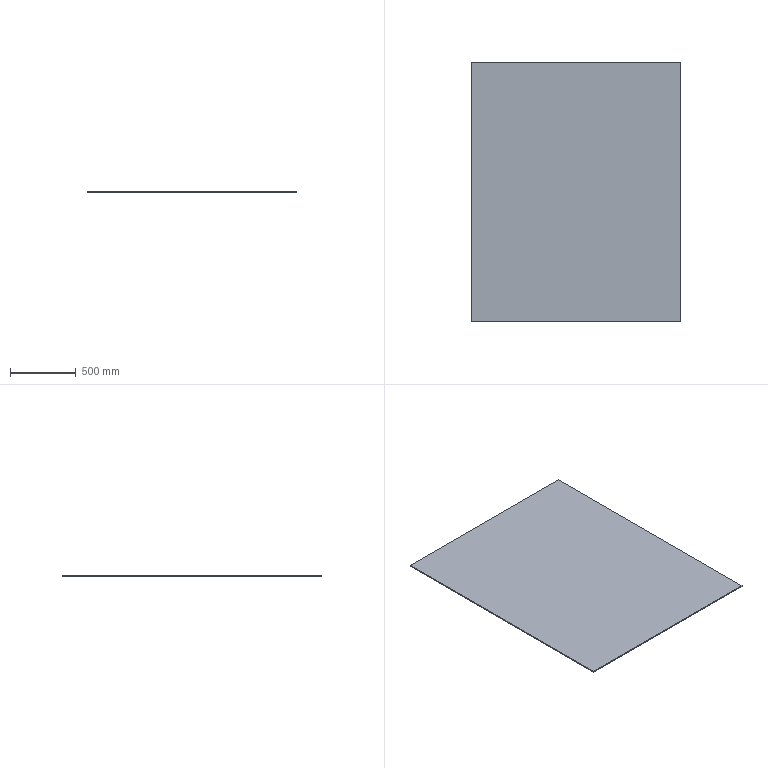Part | SolidWorks | features BaseBody 1, MoveFace 1 | 1 solid | 6 faces | box 1590 x 1968 x 8 mm | volume 25032960 mm3 | plane 6
STEP:
#1=CARTESIAN_POINT('',(0.,2.,0.));
#2=VERTEX_POINT('',#1);
#3=CARTESIAN_POINT('',(1590.,2.,0.));
#4=VERTEX_POINT('',#3);
#5=CARTESIAN_POINT('',(0.,2.,0.));
#6=DIRECTION('',(1.,0.,0.));
#7=VECTOR('',#6,1000.);
#8=LINE('',#5,#7);
#9=EDGE_CURVE('',#2,#4,#8,.T.);
#10=ORIENTED_EDGE('',*,*,#9,.F.);
#11=CARTESIAN_POINT('',(0.,1970.,0.));
#12=VERTEX_POINT('',#11);
#13=CARTESIAN_POINT('',(0.,1970.,0.));
#14=DIRECTION('',(0.,-1.,0.));
#15=VECTOR('',#14,1000.);
#16=LINE('',#13,#15);
#17=EDGE_CURVE('',#12,#2,#16,.T.);
#18=ORIENTED_EDGE('',*,*,#17,.F.);
#19=CARTESIAN_POINT('',(1590.,1970.,0.));
#20=VERTEX_POINT('',#19);
#21=CARTESIAN_POINT('',(1590.,1970.,0.));
#22=DIRECTION('',(-1.,0.,0.));
#23=VECTOR('',#22,1000.);
#24=LINE('',#21,#23);
#25=EDGE_CURVE('',#20,#12,#24,.T.);
#26=ORIENTED_EDGE('',*,*,#25,.F.);
#27=CARTESIAN_POINT('',(1590.,0.,0.));
#28=DIRECTION('',(0.,1.,0.));
#29=VECTOR('',#28,1000.);
#30=LINE('',#27,#29);
#31=EDGE_CURVE('',#4,#20,#30,.T.);
#32=ORIENTED_EDGE('',*,*,#31,.F.);
#33=EDGE_LOOP('',(#10,#18,#26,#32));
#34=FACE_OUTER_BOUND('',#33,.T.);
#35=CARTESIAN_POINT('',(795.,985.,0.));
#36=DIRECTION('',(0.,0.,1.));
#37=DIRECTION('',(1.,0.,0.));
#38=AXIS2_PLACEMENT_3D('',#35,#36,#37);
#39=PLANE('',#38);
#40=ADVANCED_FACE('',(#34),#39,.F.);
#41=CARTESIAN_POINT('',(0.,2.,8.));
#42=VERTEX_POINT('',#41);
#43=CARTESIAN_POINT('',(1590.,2.,8.));
#44=VERTEX_POINT('',#43);
#45=CARTESIAN_POINT('',(0.,2.,8.));
#46=DIRECTION('',(1.,0.,0.));
#47=VECTOR('',#46,1000.);
#48=LINE('',#45,#47);
#49=EDGE_CURVE('',#42,#44,#48,.T.);
#50=ORIENTED_EDGE('',*,*,#49,.T.);
#51=CARTESIAN_POINT('',(1590.,1970.,8.));
#52=VERTEX_POINT('',#51);
#53=CARTESIAN_POINT('',(1590.,0.,8.));
#54=DIRECTION('',(0.,1.,0.));
#55=VECTOR('',#54,1000.);
#56=LINE('',#53,#55);
#57=EDGE_CURVE('',#44,#52,#56,.T.);
#58=ORIENTED_EDGE('',*,*,#57,.T.);
#59=CARTESIAN_POINT('',(0.,1970.,8.));
#60=VERTEX_POINT('',#59);
#61=CARTESIAN_POINT('',(1590.,1970.,8.));
#62=DIRECTION('',(-1.,0.,0.));
#63=VECTOR('',#62,1000.);
#64=LINE('',#61,#63);
#65=EDGE_CURVE('',#52,#60,#64,.T.);
#66=ORIENTED_EDGE('',*,*,#65,.T.);
#67=CARTESIAN_POINT('',(0.,1970.,8.));
#68=DIRECTION('',(0.,-1.,0.));
#69=VECTOR('',#68,1000.);
#70=LINE('',#67,#69);
#71=EDGE_CURVE('',#60,#42,#70,.T.);
#72=ORIENTED_EDGE('',*,*,#71,.T.);
#73=EDGE_LOOP('',(#50,#58,#66,#72));
#74=FACE_OUTER_BOUND('',#73,.T.);
#75=CARTESIAN_POINT('',(795.,985.,8.));
#76=DIRECTION('',(0.,0.,1.));
#77=DIRECTION('',(1.,0.,0.));
#78=AXIS2_PLACEMENT_3D('',#75,#76,#77);
#79=PLANE('',#78);
#80=ADVANCED_FACE('',(#74),#79,.T.);
#81=ORIENTED_EDGE('',*,*,#9,.T.);
#82=CARTESIAN_POINT('',(1590.,2.,0.));
#83=DIRECTION('',(0.,0.,1.));
#84=VECTOR('',#83,1000.);
#85=LINE('',#82,#84);
#86=EDGE_CURVE('',#4,#44,#85,.T.);
#87=ORIENTED_EDGE('',*,*,#86,.T.);
#88=ORIENTED_EDGE('',*,*,#49,.F.);
#89=CARTESIAN_POINT('',(0.,2.,0.));
#90=DIRECTION('',(0.,0.,1.));
#91=VECTOR('',#90,1000.);
#92=LINE('',#89,#91);
#93=EDGE_CURVE('',#2,#42,#92,.T.);
#94=ORIENTED_EDGE('',*,*,#93,.F.);
#95=EDGE_LOOP('',(#81,#87,#88,#94));
#96=FACE_OUTER_BOUND('',#95,.T.);
#97=CARTESIAN_POINT('',(0.,2.,0.));
#98=DIRECTION('',(0.,-1.,0.));
#99=DIRECTION('',(0.,0.,-1.));
#100=AXIS2_PLACEMENT_3D('',#97,#98,#99);
#101=PLANE('',#100);
#102=ADVANCED_FACE('',(#96),#101,.T.);
#103=ORIENTED_EDGE('',*,*,#31,.T.);
#104=CARTESIAN_POINT('',(1590.,1970.,0.));
#105=DIRECTION('',(0.,0.,1.));
#106=VECTOR('',#105,1000.);
#107=LINE('',#104,#106);
#108=EDGE_CURVE('',#20,#52,#107,.T.);
#109=ORIENTED_EDGE('',*,*,#108,.T.);
#110=ORIENTED_EDGE('',*,*,#57,.F.);
#111=ORIENTED_EDGE('',*,*,#86,.F.);
#112=EDGE_LOOP('',(#103,#109,#110,#111));
#113=FACE_OUTER_BOUND('',#112,.T.);
#114=CARTESIAN_POINT('',(1590.,0.,0.));
#115=DIRECTION('',(1.,0.,0.));
#116=DIRECTION('',(0.,1.,0.));
#117=AXIS2_PLACEMENT_3D('',#114,#115,#116);
#118=PLANE('',#117);
#119=ADVANCED_FACE('',(#113),#118,.T.);
#120=ORIENTED_EDGE('',*,*,#25,.T.);
#121=CARTESIAN_POINT('',(0.,1970.,0.));
#122=DIRECTION('',(0.,0.,1.));
#123=VECTOR('',#122,1000.);
#124=LINE('',#121,#123);
#125=EDGE_CURVE('',#12,#60,#124,.T.);
#126=ORIENTED_EDGE('',*,*,#125,.T.);
#127=ORIENTED_EDGE('',*,*,#65,.F.);
#128=ORIENTED_EDGE('',*,*,#108,.F.);
#129=EDGE_LOOP('',(#120,#126,#127,#128));
#130=FACE_OUTER_BOUND('',#129,.T.);
#131=CARTESIAN_POINT('',(1590.,1970.,0.));
#132=DIRECTION('',(0.,1.,0.));
#133=DIRECTION('',(1.,0.,0.));
#134=AXIS2_PLACEMENT_3D('',#131,#132,#133);
#135=PLANE('',#134);
#136=ADVANCED_FACE('',(#130),#135,.T.);
#137=ORIENTED_EDGE('',*,*,#17,.T.);
#138=ORIENTED_EDGE('',*,*,#93,.T.);
#139=ORIENTED_EDGE('',*,*,#71,.F.);
#140=ORIENTED_EDGE('',*,*,#125,.F.);
#141=EDGE_LOOP('',(#137,#138,#139,#140));
#142=FACE_OUTER_BOUND('',#141,.T.);
#143=CARTESIAN_POINT('',(0.,1970.,0.));
#144=DIRECTION('',(-1.,0.,0.));
#145=DIRECTION('',(0.,1.,0.));
#146=AXIS2_PLACEMENT_3D('',#143,#144,#145);
#147=PLANE('',#146);
#148=ADVANCED_FACE('',(#142),#147,.T.);
#149=CLOSED_SHELL('',(#40,#80,#102,#119,#136,#148));
#150=MANIFOLD_SOLID_BREP('',#149);
#151=CARTESIAN_POINT('',(0.,0.,0.));
#152=DIRECTION('',(0.,0.,1.));
#153=DIRECTION('',(1.,0.,0.));
#154=AXIS2_PLACEMENT_3D('',#151,#152,#153);
#155=(LENGTH_UNIT()NAMED_UNIT(*)SI_UNIT(.MILLI.,.METRE.));
#156=UNCERTAINTY_MEASURE_WITH_UNIT(LENGTH_MEASURE(0.00001),#155,'','');
#157=(NAMED_UNIT(*)PLANE_ANGLE_UNIT()SI_UNIT($,.RADIAN.));
#158=(NAMED_UNIT(*)SI_UNIT($,.STERADIAN.)SOLID_ANGLE_UNIT());
#159=(GEOMETRIC_REPRESENTATION_CONTEXT(3)GLOBAL_UNCERTAINTY_ASSIGNED_CONTEXT((#156))GLOBAL_UNIT_ASSIGNED_CONTEXT((#155,#157,#158))REPRESENTATION_CONTEXT('',''));
#160=ADVANCED_BREP_SHAPE_REPRESENTATION('',(#150,#154),#159);